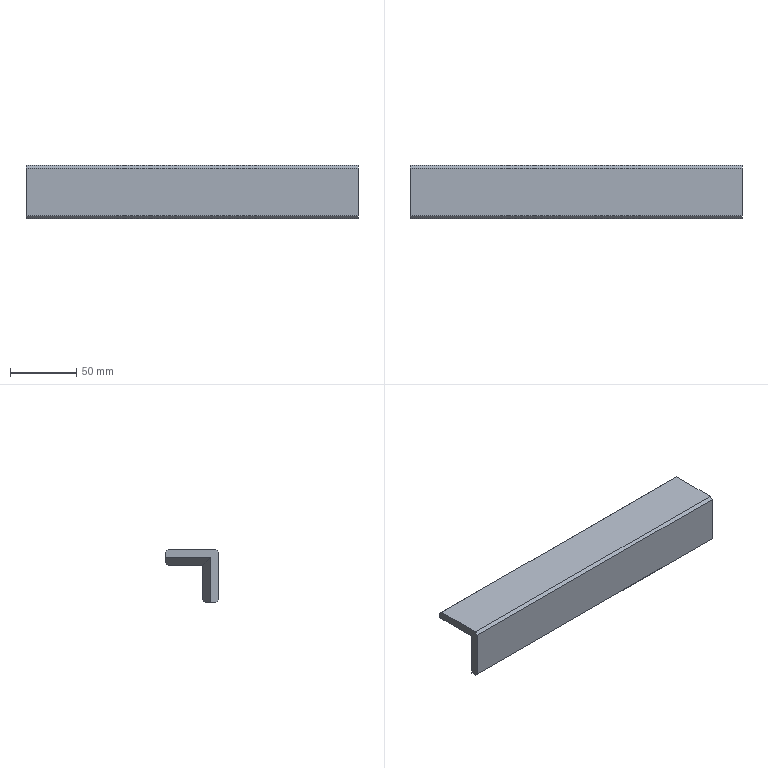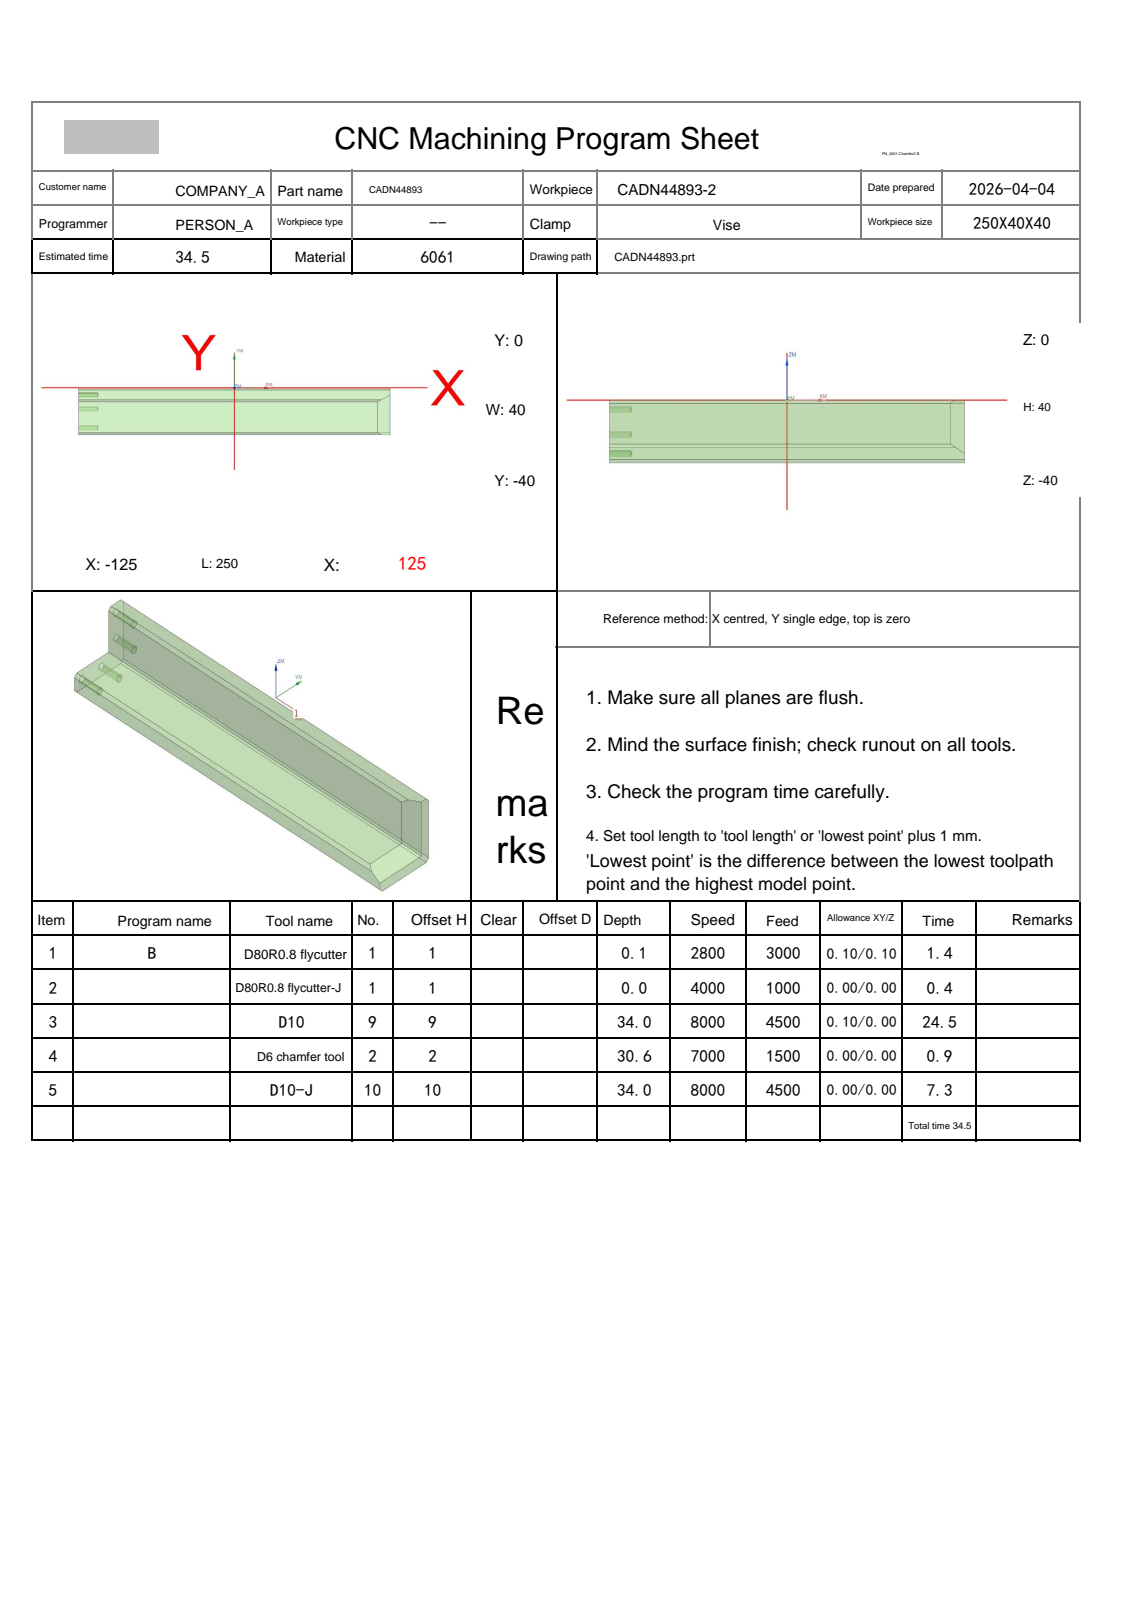NC program | NX | posted by the shop | part box 250 x 40 x 40 mm
Lines 4412 to 5961 of 8932:
N5 T10 M06
(D10-J  D=10. R=0. H=10 ce=0.40 di=0.00)
G00 G90 G54 X122. Y-40.999 M03 S7000
G43 H10 Z14.5
M08
Z-26.5
G01 Z-28. F1500.
G03 X120. Y-39. I-2. J-.001
G01 X-129.1
G02 X-130. Y-38.1 I0.0 J.9
G01 Y-35.68
G02 X-129. Y-34.68 I1. J0.0
G01 X119.1
G03 X120. Y-33.78 I0.0 J.9
G01 Y-31.36
G03 X119. Y-30.36 I-1. J0.0
G01 X-129.1
G02 X-130. Y-29.46 I0.0 J.9
G01 Y-27.04
G02 X-129. Y-26.04 I1. J0.0
G01 X119.1
G03 X120. Y-25.14 I0.0 J.9
G01 Y-22.72
G03 X119. Y-21.72 I-1. J0.0
G01 X-129.1
G02 X-130. Y-20.82 I0.0 J.9
G01 Y-18.4
G02 X-129. Y-17.4 I1. J0.0
G01 X120.
G02 X122. Y-19.399 I0.0 J-2.
G01 Z-26.5
G00 Z14.5
G00 G90 X129.655 Y-10.817 M03 S8000
Z9.5
Z-13.
G01 Z-14. F1000.
G41 D10
X129.533 Y-10.659
G03 X128.344 Y-10.074 I-1.189 J-.915
X127.572 Y-10.287 I0.0 J-1.5
G01 X117.572 Y-16.287
G02 X115. Y-17. I-2.572 J4.287
G01 X-125.
G03 X-126.49 Y-18.327 I0.0 J-1.5
G01 G40 X-126.513 Y-18.526
Z-13.
G00 Z9.5
X129.655 Y-10.817
Z-27.
G01 Z-28.
G41 D10
X129.533 Y-10.659
G03 X128.344 Y-10.074 I-1.189 J-.915
X127.572 Y-10.287 I0.0 J-1.5
G01 X117.572 Y-16.287
G02 X115. Y-17. I-2.572 J4.287
G01 X-125.
G03 X-126.49 Y-18.327 I0.0 J-1.5
G01 G40 X-126.513 Y-18.526
Z-27.
G00 Z9.5
G00 G90 X135.952 Y-5.271 M03 S7000
Z14.5
Z-27.508
G01 Z-28.008 F4500.
X128.408 Y-9.798
X127.578 Y-10.296
X120.023 Y-14.829
Y-38.008
Y-39.163
X120.022 Y-39.21
X120.034 Y-39.218 Z-28.015
X120.036 Y-39.163
Y-38.015
Y-14.821
X127.578 Y-10.296
X128.408 Y-9.798
Z-28.023
X127.578 Y-10.296
X120.049 Y-14.813
Y-38.023
Y-39.163
X120.047 Y-39.226
X120.06 Y-39.234 Z-28.031
X120.062 Y-39.163
X120.061 Y-38.031
Y-14.806
X127.578 Y-10.296
X128.408 Y-9.798
Z-28.039
X127.578 Y-10.296
X120.074 Y-14.798
Y-38.039
X120.075 Y-39.163
X120.072 Y-39.242
X120.085 Y-39.249 Z-28.046
X120.088 Y-39.163
X120.087 Y-38.046
Y-14.79
X127.578 Y-10.296
X128.408 Y-9.798
Z-28.054
X127.578 Y-10.296
X120.1 Y-14.783
Y-38.054
X120.101 Y-39.163
X120.098 Y-39.257
X120.11 Y-39.265 Z-28.062
X120.113 Y-39.163
Y-38.062
Y-14.775
X127.578 Y-10.296
X128.408 Y-9.798
Z-28.069
X127.578 Y-10.296
X120.126 Y-14.767
Y-38.069
Y-39.163
X120.123 Y-39.273
X120.136 Y-39.281 Z-28.077
X120.139 Y-39.163
Y-38.077
Y-14.759
X127.578 Y-10.296
X128.408 Y-9.798
Z-28.085
X127.578 Y-10.296
X120.151 Y-14.752
Y-38.085
X120.152 Y-39.163
X120.149 Y-39.288
X120.162 Y-39.296 Z-28.093
X120.165 Y-39.163
X120.164 Y-38.093
Y-14.744
X127.578 Y-10.296
X128.408 Y-9.798
Z-28.1
X127.578 Y-10.296
X120.177 Y-14.736
Y-38.1
X120.178 Y-39.163
X120.174 Y-39.304
X120.187 Y-39.312 Z-28.108
X120.191 Y-39.163
X120.19 Y-38.108
Y-14.729
X127.578 Y-10.296
X128.408 Y-9.798
Z-28.116
X127.578 Y-10.296
X120.203 Y-14.721
Y-38.116
Y-39.163
X120.2 Y-39.32
X120.213 Y-39.327 Z-28.123
X120.216 Y-39.163
Y-38.124
Y-14.713
X127.578 Y-10.296
X128.408 Y-9.798
Z-28.131
X127.578 Y-10.296
X120.229 Y-14.705
Y-38.131
Y-39.163
X120.226 Y-39.335
X120.239 Y-39.343 Z-28.139
X120.242 Y-39.163
Y-38.139
Y-14.698
X127.578 Y-10.296
X128.408 Y-9.798
Z-28.147
X127.578 Y-10.296
X120.254 Y-14.69
Y-38.147
X120.255 Y-39.163
X120.252 Y-39.351
X120.266 Y-39.358 Z-28.154
X120.268 Y-39.163
X120.267 Y-38.154
Y-14.682
X127.578 Y-10.296
X128.408 Y-9.798
Z-28.162
X127.578 Y-10.296
X120.28 Y-14.675
Y-38.162
X120.281 Y-39.163
X120.278 Y-39.366
X120.291 Y-39.374 Z-28.17
X120.293 Y-39.163
Y-38.17
Y-14.667
X127.578 Y-10.296
X128.408 Y-9.798
Z-28.178
X127.578 Y-10.296
X120.306 Y-14.659
Y-38.178
Y-39.163
X120.304 Y-39.382
X120.316 Y-39.39 Z-28.185
X120.319 Y-39.163
Y-38.185
Y-14.651
X127.578 Y-10.296
X128.408 Y-9.798
Z-28.193
X127.578 Y-10.296
X120.332 Y-14.644
Y-38.193
Y-39.163
X120.329 Y-39.397
X120.342 Y-39.405 Z-28.201
X120.344 Y-38.201
Y-14.636
X127.578 Y-10.296
X128.408 Y-9.798
Z-28.208
X127.578 Y-10.296
X120.357 Y-14.628
Y-38.208
X120.355 Y-39.413
X120.368 Y-39.421 Z-28.216
X120.37 Y-38.216
Y-14.621
X127.578 Y-10.296
X128.408 Y-9.798
Z-28.224
X127.578 Y-10.296
X120.383 Y-14.613
Y-38.224
X120.381 Y-39.429
X120.394 Y-39.436 Z-28.232
X120.396 Y-38.232
Y-14.605
X127.578 Y-10.296
X128.408 Y-9.798
Z-28.239
X127.578 Y-10.296
X120.409 Y-14.597
Y-38.239
X120.407 Y-39.444
X120.42 Y-39.452 Z-28.247
X120.422 Y-38.247
Y-14.59
X127.578 Y-10.296
X128.408 Y-9.798
Z-28.255
X127.578 Y-10.296
X120.434 Y-14.582
Y-38.255
X120.432 Y-39.46
X120.445 Y-39.468 Z-28.262
X120.447 Y-38.262
Y-14.574
X127.578 Y-10.296
X128.408 Y-9.798
Z-28.27
X127.578 Y-10.296
X120.46 Y-14.567
Y-38.27
X120.458 Y-39.475
X120.471 Y-39.483 Z-28.278
X120.473 Y-38.278
Y-14.559
X127.578 Y-10.296
X128.408 Y-9.798
Z-28.286
X127.578 Y-10.296
X120.486 Y-14.551
Y-38.286
X120.484 Y-39.491
X120.497 Y-39.499 Z-28.293
X120.499 Y-38.293
Y-14.543
X127.578 Y-10.296
X128.408 Y-9.798
Z-28.301
X127.578 Y-10.296
X120.512 Y-14.536
Y-38.301
X120.51 Y-39.506
X120.523 Y-39.514 Z-28.309
X120.524 Y-38.309
Y-14.528
X127.578 Y-10.296
X128.408 Y-9.798
Z-28.316
X127.578 Y-10.296
X120.537 Y-14.52
Y-38.316
X120.536 Y-39.522
X120.549 Y-39.53 Z-28.324
X120.55 Y-38.324
Y-14.512
X127.578 Y-10.296
X128.408 Y-9.798
Z-28.332
X127.578 Y-10.296
X120.563 Y-14.505
Y-38.332
X120.562 Y-39.538
X120.575 Y-39.545 Z-28.34
X120.576 Y-38.34
Y-14.497
X127.578 Y-10.296
X128.408 Y-9.798
Z-28.347
X127.578 Y-10.296
X120.589 Y-14.489
Y-38.347
X120.588 Y-39.553
X120.601 Y-39.561 Z-28.355
X120.602 Y-38.355
Y-14.482
X127.578 Y-10.296
X128.408 Y-9.798
Z-28.363
X127.578 Y-10.296
X120.615 Y-14.474
Y-38.363
X120.614 Y-39.569
X120.627 Y-39.577 Z-28.37
Y-38.37
Y-14.466
X127.578 Y-10.296
X128.408 Y-9.798
Z-28.378
X127.578 Y-10.296
X120.64 Y-14.458
Y-38.378
Y-39.584
X120.653 Y-39.592 Z-28.386
Y-38.386
Y-14.451
X127.578 Y-10.296
X128.408 Y-9.798
Z-28.394
X127.578 Y-10.296
X120.666 Y-14.443
Y-38.394
Y-39.6
X120.679 Y-39.608 Z-28.401
Y-38.401
Y-14.435
X127.578 Y-10.296
X128.408 Y-9.798
Z-28.409
X127.578 Y-10.296
X120.692 Y-14.428
Y-38.409
Y-39.615
X120.704 Y-39.623 Z-28.417
X120.705 Y-38.417
Y-14.42
X127.578 Y-10.296
X128.408 Y-9.798
Z-28.424
X127.578 Y-10.296
X120.717 Y-14.412
Y-38.424
Y-39.631
X120.73 Y-39.639 Z-28.432
X120.731 Y-39.61
X120.73 Y-38.432
Y-14.404
X127.578 Y-10.296
X128.408 Y-9.798
Z-28.44
X127.578 Y-10.296
X120.743 Y-14.397
Y-38.44
X120.744 Y-39.61
X120.742 Y-39.646
X120.755 Y-39.654 Z-28.448
X120.756 Y-39.61
Y-38.448
Y-14.389
X127.578 Y-10.296
X128.408 Y-9.798
Z-28.455
X127.578 Y-10.296
X120.769 Y-14.381
Y-38.455
Y-39.61
X120.767 Y-39.662
X120.78 Y-39.669 Z-28.463
X120.782 Y-39.61
Y-38.463
Y-14.374
X127.578 Y-10.296
X128.408 Y-9.798
Z-28.471
X127.578 Y-10.296
X120.795 Y-14.366
Y-38.471
Y-39.61
X120.793 Y-39.677
X120.805 Y-39.685 Z-28.478
X120.808 Y-39.61
X120.807 Y-38.479
Y-14.358
X127.578 Y-10.296
X128.408 Y-9.798
Z-28.486
X127.578 Y-10.296
X120.82 Y-14.35
Y-38.486
X120.821 Y-39.61
X120.818 Y-39.692
X120.831 Y-39.7 Z-28.494
X120.834 Y-39.61
X120.833 Y-38.494
Y-14.343
X127.578 Y-10.296
X128.408 Y-9.798
Z-28.502
X127.578 Y-10.296
X120.846 Y-14.335
Y-38.502
Y-39.61
X120.844 Y-39.708
X120.856 Y-39.716 Z-28.509
X120.859 Y-39.61
Y-38.509
Y-14.327
X127.578 Y-10.296
X128.408 Y-9.798
Z-28.517
X127.578 Y-10.296
X120.872 Y-14.32
Y-38.517
Y-39.61
X120.869 Y-39.723
X120.882 Y-39.731 Z-28.525
X120.885 Y-39.61
Y-38.525
Y-14.312
X127.578 Y-10.296
X128.408 Y-9.798
Z-28.533
X127.578 Y-10.296
X120.898 Y-14.304
Y-38.533
Y-39.61
X120.895 Y-39.739
X120.907 Y-39.746 Z-28.54
X120.911 Y-39.61
X120.91 Y-38.54
Y-14.296
X127.578 Y-10.296
X128.408 Y-9.798
Z-28.548
X127.578 Y-10.296
X120.923 Y-14.289
Y-38.548
X120.924 Y-39.61
X120.92 Y-39.754
X120.933 Y-39.762 Z-28.556
X120.936 Y-39.61
Y-38.556
Y-14.281
X127.578 Y-10.296
X128.408 Y-9.798
Z-28.563
X127.578 Y-10.296
X120.949 Y-14.273
Y-38.563
Y-39.61
X120.946 Y-39.769
X120.959 Y-39.777 Z-28.571
X120.962 Y-39.61
Y-38.571
Y-14.266
X127.578 Y-10.296
X128.408 Y-9.798
Z-28.579
X127.578 Y-10.296
X120.975 Y-14.258
Y-38.579
Y-39.61
X120.972 Y-39.785
X120.984 Y-39.792 Z-28.587
X120.988 Y-39.61
Y-38.587
Y-14.25
X127.578 Y-10.296
X128.408 Y-9.798
Z-28.594
X127.578 Y-10.296
X121. Y-14.242
Y-38.594
X121.001 Y-39.61
X120.997 Y-39.8
X121.01 Y-39.808 Z-28.602
X121.014 Y-39.61
X121.013 Y-38.602
Y-14.235
X127.578 Y-10.296
X128.408 Y-9.798
Z-28.61
X127.578 Y-10.296
X121.026 Y-14.227
Y-38.61
X121.027 Y-39.61
X121.023 Y-39.816
X121.036 Y-39.823 Z-28.617
X121.039 Y-39.61
Y-38.617
Y-14.219
X127.578 Y-10.296
X128.408 Y-9.798
Z-28.625
X127.578 Y-10.296
X121.052 Y-14.212
Y-38.625
Y-39.61
X121.049 Y-39.831
X121.062 Y-39.839 Z-28.633
X121.065 Y-39.61
Y-38.633
Y-14.204
X127.578 Y-10.296
X128.408 Y-9.798
Z-28.641
X127.578 Y-10.296
X121.078 Y-14.196
Y-38.641
Y-39.61
X121.075 Y-39.846
X121.088 Y-39.854 Z-28.648
X121.09 Y-38.648
Y-14.188
X127.578 Y-10.296
X128.408 Y-9.798
Z-28.656
X127.578 Y-10.296
X121.103 Y-14.181
Y-38.656
X121.101 Y-39.862
X121.114 Y-39.869 Z-28.664
X121.116 Y-38.664
Y-14.173
X127.578 Y-10.296
X128.408 Y-9.798
Z-28.671
X127.578 Y-10.296
X121.129 Y-14.165
Y-38.671
X121.127 Y-39.877
X121.14 Y-39.885 Z-28.679
X121.142 Y-38.679
Y-14.157
X127.578 Y-10.296
X128.408 Y-9.798
Z-28.687
X127.578 Y-10.296
X121.155 Y-14.15
Y-38.687
X121.153 Y-39.893
X121.166 Y-39.9 Z-28.695
X121.168 Y-38.695
Y-14.142
X127.578 Y-10.296
X128.408 Y-9.798
Z-28.702
X127.578 Y-10.296
X121.18 Y-14.134
Y-38.702
X121.179 Y-39.908
X121.192 Y-39.916 Z-28.71
X121.193 Y-38.71
Y-14.127
X127.578 Y-10.296
X128.408 Y-9.798
Z-28.718
X127.578 Y-10.296
X121.206 Y-14.119
Y-38.718
X121.205 Y-39.923
X121.218 Y-39.931 Z-28.725
X121.219 Y-38.725
Y-14.111
X127.578 Y-10.296
X128.408 Y-9.798
Z-28.733
X127.578 Y-10.296
X121.232 Y-14.103
Y-38.733
X121.231 Y-39.939
X121.244 Y-39.946 Z-28.741
X121.245 Y-38.741
Y-14.096
X127.578 Y-10.296
X128.408 Y-9.798
Z-28.749
X127.578 Y-10.296
X121.258 Y-14.088
Y-38.749
X121.257 Y-39.954
X121.27 Y-39.962 Z-28.756
X121.271 Y-38.756
Y-14.08
X127.578 Y-10.296
X128.408 Y-9.798
Z-28.764
X127.578 Y-10.296
X121.283 Y-14.073
Y-38.764
Y-39.97
X121.296 Y-39.977 Z-28.772
Y-38.772
Y-14.065
X127.578 Y-10.296
X128.408 Y-9.798
Z-28.779
X127.578 Y-10.296
X121.309 Y-14.057
Y-38.779
Y-39.985
X121.321 Y-39.993 Z-28.787
X121.322 Y-38.787
Y-14.049
X127.578 Y-10.296
X128.408 Y-9.798
Z-28.795
X127.578 Y-10.296
X121.335 Y-14.042
Y-38.795
X121.334 Y-40.
X121.347 Y-40.008 Z-28.803
X121.348 Y-38.803
Y-14.034
X127.578 Y-10.296
X128.408 Y-9.798
Z-28.81
X127.578 Y-10.296
X121.361 Y-14.026
Y-38.81
X121.36 Y-40.016
X121.373 Y-40.023 Z-28.818
Y-38.818
Y-14.019
X127.578 Y-10.296
X128.408 Y-9.798
Z-28.826
X127.578 Y-10.296
X121.386 Y-14.011
Y-38.826
Y-40.031
X121.399 Y-40.039 Z-28.833
Y-38.834
Y-14.003
X127.578 Y-10.296
X128.408 Y-9.798
Z-28.841
X127.578 Y-10.296
X121.412 Y-13.995
Y-38.841
Y-40.047
X121.425 Y-40.054 Z-28.849
Y-38.849
Y-13.988
X127.578 Y-10.296
X128.408 Y-9.798
Z-28.857
X127.578 Y-10.296
X121.438 Y-13.98
Y-38.857
Y-40.062
X121.45 Y-40.07 Z-28.864
X121.451 Y-38.864
Y-13.972
X127.578 Y-10.296
X128.408 Y-9.798
Z-28.872
X127.578 Y-10.296
X121.463 Y-13.965
Y-38.872
Y-40.077
X121.476 Y-40.085 Z-28.88
X121.477 Y-40.057
X121.476 Y-38.88
Y-13.957
X127.578 Y-10.296
X128.408 Y-9.798
Z-28.888
X127.578 Y-10.296
X121.489 Y-13.949
Y-38.888
X121.49 Y-40.057
X121.488 Y-40.093
X121.501 Y-40.1 Z-28.895
X121.502 Y-40.057
Y-38.895
Y-13.941
X127.578 Y-10.296
X128.408 Y-9.798
Z-28.903
X127.578 Y-10.296
X121.515 Y-13.934
Y-38.903
Y-40.057
X121.513 Y-40.108
X121.526 Y-40.116 Z-28.911
X121.528 Y-40.057
Y-38.911
Y-13.926
X127.578 Y-10.296
X128.408 Y-9.798
Z-28.918
X127.578 Y-10.296
X121.541 Y-13.918
Y-38.918
Y-40.057
X121.539 Y-40.123
X121.551 Y-40.131 Z-28.926
X121.554 Y-40.057
X121.553 Y-38.926
Y-13.911
X127.578 Y-10.296
X128.408 Y-9.798
Z-28.934
X127.578 Y-10.296
X121.566 Y-13.903
Y-38.934
X121.567 Y-40.057
X121.564 Y-40.139
X121.577 Y-40.147 Z-28.942
X121.58 Y-40.057
X121.579 Y-38.942
Y-13.895
X127.578 Y-10.296
X128.408 Y-9.798
Z-28.949
X127.578 Y-10.296
X121.592 Y-13.887
Y-38.949
Y-40.057
X121.59 Y-40.154
X121.603 Y-40.162 Z-28.957
X121.605 Y-40.057
Y-38.957
Y-13.88
X127.578 Y-10.296
X128.408 Y-9.798
Z-28.965
X127.578 Y-10.296
X121.618 Y-13.872
Y-38.965
Y-40.057
X121.615 Y-40.17
X121.628 Y-40.177 Z-28.972
X121.631 Y-40.057
Y-38.972
Y-13.864
X127.578 Y-10.296
X128.408 Y-9.798
Z-28.98
X127.578 Y-10.296
X121.644 Y-13.857
Y-38.98
Y-40.057
X121.641 Y-40.185
X121.654 Y-40.192 Z-28.988
X121.657 Y-40.057
X121.656 Y-38.988
Y-13.849
X127.578 Y-10.296
X128.408 Y-9.798
Z-28.996
X127.578 Y-10.296
X121.669 Y-13.841
Y-38.996
X121.67 Y-40.057
X121.666 Y-40.2
X121.679 Y-40.208 Z-29.003
X121.682 Y-40.057
Y-39.003
Y-13.833
X127.578 Y-10.296
X128.408 Y-9.798
Z-29.011
X127.578 Y-10.296
X121.695 Y-13.826
Y-39.011
Y-40.057
X121.692 Y-40.215
X121.705 Y-40.223 Z-29.019
X121.708 Y-40.057
Y-39.019
Y-13.818
X127.578 Y-10.296
X128.408 Y-9.798
Z-29.026
X127.578 Y-10.296
X121.721 Y-13.81
Y-39.026
Y-40.057
X121.718 Y-40.231
X121.731 Y-40.238 Z-29.034
X121.734 Y-40.057
Y-39.034
Y-13.802
X127.578 Y-10.296
X128.408 Y-9.798
Z-29.042
X127.578 Y-10.296
X121.746 Y-13.795
Y-39.042
X121.747 Y-40.057
X121.743 Y-40.246
X121.756 Y-40.254 Z-29.05
X121.76 Y-40.057
X121.759 Y-39.05
Y-13.787
X127.578 Y-10.296
X128.408 Y-9.798
Z-29.057
X127.578 Y-10.296
X121.772 Y-13.779
Y-39.057
X121.773 Y-40.057
X121.769 Y-40.261
X121.782 Y-40.269 Z-29.065
X121.785 Y-40.057
Y-39.065
Y-13.772
X127.578 Y-10.296
X128.408 Y-9.798
Z-29.073
X127.578 Y-10.296
X121.798 Y-13.764
Y-39.073
Y-40.057
X121.795 Y-40.277
X121.808 Y-40.284 Z-29.08
X121.811 Y-40.057
Y-39.08
Y-13.756
X127.578 Y-10.296
X128.408 Y-9.798
Z-29.088
X127.578 Y-10.296
X121.824 Y-13.748
Y-39.088
Y-40.057
X121.821 Y-40.292
X121.834 Y-40.3 Z-29.096
X121.836 Y-39.096
Y-13.741
X127.578 Y-10.296
X128.408 Y-9.798
Z-29.104
X127.578 Y-10.296
X121.849 Y-13.733
Y-39.104
X121.847 Y-40.307
X121.86 Y-40.315 Z-29.111
X121.862 Y-39.111
Y-13.725
X127.578 Y-10.296
X128.408 Y-9.798
Z-29.119
X127.578 Y-10.296
X121.875 Y-13.718
Y-39.119
X121.873 Y-40.323
X121.886 Y-40.33 Z-29.127
X121.888 Y-39.127
Y-13.71
X127.578 Y-10.296
X128.408 Y-9.798
Z-29.134
X127.578 Y-10.296
X121.901 Y-13.702
Y-39.134
X121.899 Y-40.338
X121.912 Y-40.345 Z-29.142
X121.914 Y-39.142
Y-13.694
X127.578 Y-10.296
X128.408 Y-9.798
Z-29.15
X127.578 Y-10.296
X121.926 Y-13.687
Y-39.15
X121.925 Y-40.353
X121.938 Y-40.361 Z-29.158
X121.939 Y-39.158
Y-13.679
X127.578 Y-10.296
X128.408 Y-9.798
Z-29.165
X127.578 Y-10.296
X121.952 Y-13.671
Y-39.165
X121.951 Y-40.368
X121.964 Y-40.376 Z-29.173
X121.965 Y-39.173
Y-13.664
X127.578 Y-10.296
X128.408 Y-9.798
Z-29.181
X127.578 Y-10.296
X121.978 Y-13.656
Y-39.181
X121.977 Y-40.384
X121.99 Y-40.391 Z-29.188
X121.991 Y-39.189
Y-13.648
X127.578 Y-10.296
X128.408 Y-9.798
Z-29.196
X127.578 Y-10.296
X122.004 Y-13.64
Y-39.196
X122.003 Y-40.399
X122.016 Y-40.407 Z-29.204
X122.017 Y-39.204
Y-13.633
X127.578 Y-10.296
X128.408 Y-9.798
Z-29.212
X127.578 Y-10.296
X122.029 Y-13.625
Y-39.212
Y-40.414
X122.042 Y-40.422 Z-29.219
Y-39.219
Y-13.617
X127.578 Y-10.296
X128.408 Y-9.798
Z-29.227
X127.578 Y-10.296
X122.055 Y-13.61
Y-39.227
Y-40.43
X122.068 Y-40.437 Z-29.235
Y-39.235
Y-13.602
X127.578 Y-10.296
X128.408 Y-9.798
Z-29.243
X127.578 Y-10.296
X122.081 Y-13.594
Y-39.243
Y-40.445
X122.094 Y-40.452 Z-29.25
Y-39.25
Y-13.586
X127.578 Y-10.296
X128.408 Y-9.798
Z-29.258
X127.578 Y-10.296
X122.107 Y-13.579
Y-39.258
Y-40.46
X122.12 Y-40.468 Z-29.266
X122.119 Y-39.266
Y-13.571
X127.578 Y-10.296
X128.408 Y-9.798
Z-29.273
X127.578 Y-10.296
X122.132 Y-13.563
Y-39.273
Y-40.475
X122.145 Y-40.483 Z-29.281
Y-39.281
Y-13.556
X127.578 Y-10.296
X128.408 Y-9.798
Z-29.289
X127.578 Y-10.296
X122.158 Y-13.548
Y-39.289
Y-40.49
X122.171 Y-40.498 Z-29.297
Y-39.297
Y-13.54
X127.578 Y-10.296
X128.408 Y-9.798
Z-29.304
X127.578 Y-10.296
X122.184 Y-13.532
Y-39.304
Y-40.506
X122.197 Y-40.513 Z-29.312
Y-39.312
Y-13.525
X127.578 Y-10.296
X128.408 Y-9.798
Z-29.32
X127.578 Y-10.296
X122.209 Y-13.517
Y-39.32
Y-40.521
X122.222 Y-40.528 Z-29.327
X122.223 Y-40.505
X122.222 Y-39.327
Y-13.509
X127.578 Y-10.296
X128.408 Y-9.798
Z-29.335
X127.578 Y-10.296
X122.235 Y-13.501
Y-39.335
X122.236 Y-40.505
X122.234 Y-40.536
X122.247 Y-40.543 Z-29.343
X122.248 Y-40.505
Y-39.343
Y-13.494
X127.578 Y-10.296
X128.408 Y-9.798
Z-29.351
X127.578 Y-10.296
X122.261 Y-13.486
Y-39.351
Y-40.505
X122.259 Y-40.551
X122.272 Y-40.559 Z-29.358
X122.274 Y-40.505
Y-39.358
Y-13.478
X127.578 Y-10.296
X128.408 Y-9.798
Z-29.366
X127.578 Y-10.296
X122.287 Y-13.471
Y-39.366
Y-40.505
X122.285 Y-40.566
X122.297 Y-40.574 Z-29.374
X122.3 Y-40.505
Y-39.374
Y-13.463
X127.578 Y-10.296
X128.408 Y-9.798
Z-29.381
X127.578 Y-10.296
X122.312 Y-13.455
Y-39.381
X122.313 Y-40.505
X122.31 Y-40.581
X122.323 Y-40.589 Z-29.389
X122.326 Y-40.505
X122.325 Y-39.389
Y-13.447
X127.578 Y-10.296
X128.408 Y-9.798
Z-29.397
X127.578 Y-10.296
X122.338 Y-13.44
Y-39.397
Y-40.505
X122.336 Y-40.597
X122.348 Y-40.604 Z-29.405
X122.351 Y-40.505
Y-39.405
Y-13.432
X127.578 Y-10.296
X128.408 Y-9.798
Z-29.412
X127.578 Y-10.296
X122.364 Y-13.424
Y-39.412
Y-40.505
X122.361 Y-40.612
X122.374 Y-40.619 Z-29.42
X122.377 Y-40.505
Y-39.42
Y-13.417
X127.578 Y-10.296
X128.408 Y-9.798
Z-29.428
X127.578 Y-10.296
X122.39 Y-13.409
Y-39.428
Y-40.505
X122.387 Y-40.627
X122.4 Y-40.635 Z-29.435
X122.403 Y-40.505
X122.402 Y-39.435
Y-13.401
X127.578 Y-10.296
X128.408 Y-9.798
Z-29.443
X127.578 Y-10.296
X122.415 Y-13.393
Y-39.443
X122.416 Y-40.505
X122.412 Y-40.642
X122.425 Y-40.65 Z-29.451
X122.428 Y-40.505
Y-39.451
Y-13.386
X127.578 Y-10.296
X128.408 Y-9.798
Z-29.459
X127.578 Y-10.296
X122.441 Y-13.378
Y-39.459
Y-40.505
X122.438 Y-40.657
X122.451 Y-40.665 Z-29.466
X122.454 Y-40.505
Y-39.466
Y-13.37
X127.578 Y-10.296
X128.408 Y-9.798
Z-29.474
X127.578 Y-10.296
X122.467 Y-13.363
Y-39.474
Y-40.505
X122.464 Y-40.673
X122.479 Y-40.68 Z-29.482
X122.48 Y-39.482
Y-13.355
X127.578 Y-10.296
X128.408 Y-9.798
Z-29.489
X127.578 Y-10.296
X122.492 Y-13.347
Y-39.489
X122.493 Y-40.505
X122.49 Y-40.688
X122.503 Y-40.695 Z-29.497
X122.506 Y-40.505
X122.505 Y-39.497
Y-13.339
X127.578 Y-10.296
X128.408 Y-9.798
Z-29.505
X127.578 Y-10.296
X122.518 Y-13.332
Y-39.505
Y-40.505
X122.516 Y-40.703
X122.528 Y-40.711 Z-29.513
X122.531 Y-40.505
Y-39.513
Y-13.324
X127.578 Y-10.296
X128.408 Y-9.798
Z-29.52
X127.578 Y-10.296
X122.544 Y-13.316
Y-39.52
Y-40.505
X122.541 Y-40.718
X122.554 Y-40.726 Z-29.528
X122.557 Y-40.505
Y-39.528
Y-13.309
X127.578 Y-10.296
X128.408 Y-9.798
Z-29.536
X127.578 Y-10.296
X122.57 Y-13.301
Y-39.536
Y-40.505
X122.567 Y-40.733
X122.58 Y-40.741 Z-29.543
X122.583 Y-40.505
X122.582 Y-39.544
Y-13.293
X127.578 Y-10.296
X128.408 Y-9.798
Z-29.551
X127.578 Y-10.296
X122.595 Y-13.285
Y-39.551
X122.593 Y-40.749
X122.606 Y-40.756 Z-29.559
X122.608 Y-39.559
Y-13.278
X127.578 Y-10.296
X128.408 Y-9.798
Z-29.567
X127.578 Y-10.296
X122.621 Y-13.27
Y-39.567
X122.618 Y-40.764
X122.631 Y-40.772 Z-29.574
X122.634 Y-39.574
Y-13.262
X127.578 Y-10.296
X128.408 Y-9.798
Z-29.582
X127.578 Y-10.296
X122.647 Y-13.255
Y-39.582
X122.644 Y-40.779
X122.657 Y-40.787 Z-29.59
X122.66 Y-39.59
Y-13.247
X127.578 Y-10.296
X128.408 Y-9.798
Z-29.598
X127.578 Y-10.296
X122.673 Y-13.239
Y-39.598
X122.67 Y-40.794
X122.683 Y-40.802 Z-29.605
X122.685 Y-39.605
Y-13.231
X127.578 Y-10.296
X128.408 Y-9.798
Z-29.613
X127.578 Y-10.296
X122.698 Y-13.224
Y-39.613
X122.696 Y-40.81
X122.709 Y-40.817 Z-29.621
X122.711 Y-39.621
Y-13.216
X127.578 Y-10.296
X128.408 Y-9.798
Z-29.628
X127.578 Y-10.296
X122.724 Y-13.208
Y-39.628
X122.722 Y-40.825
X122.735 Y-40.832 Z-29.636
X122.737 Y-39.636
Y-13.201
X127.578 Y-10.296
X128.408 Y-9.798
Z-29.644
X127.578 Y-10.296
X122.75 Y-13.193
Y-39.644
X122.748 Y-40.84
X122.761 Y-40.848 Z-29.652
X122.763 Y-39.652
Y-13.185
X127.578 Y-10.296
X128.408 Y-9.798
Z-29.659
X127.578 Y-10.296
X122.775 Y-13.177
Y-39.659
X122.774 Y-40.855
X122.787 Y-40.863 Z-29.667
X122.788 Y-39.667
Y-13.17
X127.578 Y-10.296
X128.408 Y-9.798
Z-29.675
X127.578 Y-10.296
X122.801 Y-13.162
Y-39.675
X122.8 Y-40.87
X122.813 Y-40.878 Z-29.682
X122.814 Y-39.682
Y-13.154
X127.578 Y-10.296
X128.408 Y-9.798
Z-29.69
X127.578 Y-10.296
X122.827 Y-13.146
Y-39.69
X122.826 Y-40.886
X122.839 Y-40.893 Z-29.698
X122.84 Y-39.698
Y-13.139
X127.578 Y-10.296
X128.408 Y-9.798
Z-29.706
X127.578 Y-10.296
X122.853 Y-13.131
Y-39.706
X122.852 Y-40.901
X122.865 Y-40.908 Z-29.713
Y-39.713
Y-13.123
X127.578 Y-10.296
X128.408 Y-9.798
Z-29.721
X127.578 Y-10.296
X122.878 Y-13.116
Y-39.721
Y-40.916
X122.891 Y-40.924 Z-29.729
Y-39.729
Y-13.108
X127.578 Y-10.296
X128.408 Y-9.798
Z-29.736
X127.578 Y-10.296
X122.904 Y-13.1
Y-39.736
Y-40.931
X122.917 Y-40.939 Z-29.744
Y-39.744
Y-13.092
X127.578 Y-10.296
X128.408 Y-9.798
Z-29.752
X127.578 Y-10.296
X122.93 Y-13.085
Y-39.752
Y-40.946
X122.943 Y-40.953 Z-29.76
Y-39.76
Y-13.077
X127.578 Y-10.296
X128.408 Y-9.798
Z-29.767
X127.578 Y-10.296
X122.955 Y-13.069
Y-39.767
X122.956 Y-40.956
X122.968 Y-40.959 Z-29.775
Y-39.775
Y-13.062
X127.578 Y-10.296
X128.408 Y-9.798
Z-29.783
X127.578 Y-10.296
X122.981 Y-13.054
Y-39.783
Y-40.963
X122.994 Y-40.966 Z-29.79
Y-39.79
Y-13.046
X127.578 Y-10.296
X128.408 Y-9.798
Z-29.798
X127.578 Y-10.296
X123.007 Y-13.038
Y-39.798
X123.006 Y-40.97
X123.019 Y-40.973 Z-29.806
X123.02 Y-39.806
Y-13.031
X127.578 Y-10.296
X128.408 Y-9.798
Z-29.814
X127.578 Y-10.296
X123.033 Y-13.023
Y-39.814
X123.032 Y-40.976
X123.045 Y-40.98 Z-29.821
X123.046 Y-40.952
Y-39.821
Y-13.015
X127.578 Y-10.296
X128.408 Y-9.798
Z-29.829
X127.578 Y-10.296
X123.058 Y-13.008
Y-39.829
X123.059 Y-40.952
X123.057 Y-40.983
X123.07 Y-40.986 Z-29.837
X123.071 Y-40.952
Y-39.837
Y-13.
X127.578 Y-10.296
X128.408 Y-9.798
Z-29.844
X127.578 Y-10.296
X123.084 Y-12.992
Y-39.844
Y-40.952
X123.083 Y-40.99
X123.096 Y-40.993 Z-29.852
X123.097 Y-40.952
Y-39.852
Y-12.984
X127.578 Y-10.296
X128.408 Y-9.798
Z-29.86
X127.578 Y-10.296
X123.11 Y-12.977
Y-39.86
Y-40.952
X123.108 Y-40.996
X123.121 Y-41. Z-29.868
X123.123 Y-40.952
Y-39.868
Y-12.969
X127.578 Y-10.296
X128.408 Y-9.798
Z-29.875
X127.578 Y-10.296
X123.136 Y-12.961
Y-39.875
Y-40.952
X123.134 Y-41.003
X123.147 Y-41.006 Z-29.883
X123.149 Y-40.952
X123.148 Y-39.883
Y-12.954
X127.578 Y-10.296
X128.408 Y-9.798
Z-29.891
X127.578 Y-10.296
X123.161 Y-12.946
Y-39.891
X123.162 Y-40.952
X123.16 Y-41.01
X123.172 Y-41.013 Z-29.898
X123.174 Y-40.952
Y-39.899
Y-12.938
X127.578 Y-10.296
X128.408 Y-9.798
Z-29.906
X127.578 Y-10.296
X123.187 Y-12.93
Y-39.906
Y-40.952
X123.185 Y-41.016
X123.198 Y-41.02 Z-29.914
X123.2 Y-40.952
Y-39.914
Y-12.923
X127.578 Y-10.296
X128.408 Y-9.798
Z-29.922
X127.578 Y-10.296
X123.213 Y-12.915
Y-39.922
Y-40.952
X123.211 Y-41.023
X123.223 Y-41.026 Z-29.929
X123.226 Y-40.952
Y-39.929
Y-12.907
X127.578 Y-10.296
X128.408 Y-9.798
Z-29.937
X127.578 Y-10.296
X123.238 Y-12.9
Y-39.937
X123.239 Y-40.952
X123.236 Y-41.03
X123.249 Y-41.033 Z-29.945
X123.252 Y-40.952
X123.251 Y-39.945
Y-12.892
X127.578 Y-10.296
X128.408 Y-9.798
Z-29.953
X127.578 Y-10.296
X123.264 Y-12.884
Y-39.953
Y-40.952
X123.262 Y-41.036
X123.271 Y-41.039 Z-29.956
X123.275 Y-41.04 Z-29.96
X123.277 Y-40.952
Y-39.96
Y-12.876
X127.578 Y-10.296
X128.408 Y-9.798
Z-29.968
X127.578 Y-10.296
X123.29 Y-12.869
Y-39.968
Y-40.952
X123.287 Y-41.043
X123.297 Y-41.045 Z-29.972
X123.3 Y-41.046 Z-29.976
X123.303 Y-40.952
Y-39.976
Y-12.861
X127.578 Y-10.296
X128.408 Y-9.798
Z-29.983
X127.578 Y-10.296
X123.316 Y-12.853
Y-39.983
Y-40.952
X123.313 Y-41.05
X123.322 Y-41.052 Z-29.987
X123.326 Y-41.053 Z-29.991
X123.329 Y-40.952
X123.328 Y-39.991
Y-12.846
X127.578 Y-10.296
X128.408 Y-9.798
Z-29.999
X127.578 Y-10.296
X123.341 Y-12.838
Y-39.999
X123.342 Y-40.952
X123.339 Y-41.056
X123.348 Y-41.059 Z-30.003
X123.352 Y-41.06 Z-30.007
X123.354 Y-40.952
Y-40.
Y-12.83
X127.578 Y-10.296
X128.408 Y-9.798
Z-30.014
X127.578 Y-10.296
X123.367 Y-12.822
Y-40.
Y-40.952
X123.366 Y-41.062
X123.374 Z-30.018
X123.377 Z-30.022
X123.38 Y-40.952
Y-40.
Y-12.815
X127.578 Y-10.296
X128.408 Y-9.798
Z-30.03
X127.578 Y-10.296
X123.393 Y-12.807
Y-40.
Y-40.952
X123.39 Y-41.063
X123.399 Z-30.034
X123.403 Z-30.037
X123.406 Y-40.952
Y-40.
Y-12.799
X127.578 Y-10.296
X128.408 Y-9.798
Z-30.045
X127.578 Y-10.296
X123.419 Y-12.791
Y-40.
Y-40.952
X123.416 Y-41.063
X123.425 Z-30.049
X123.429 Z-30.053
X123.432 Y-40.952
X123.431 Y-40.
Y-12.784
X127.578 Y-10.296
X128.408 Y-9.798
Z-30.061
X127.578 Y-10.296
X123.444 Y-12.776
Y-40.
Y-40.952
X123.442 Y-41.063
X123.451 Z-30.064
X123.455 Z-30.068